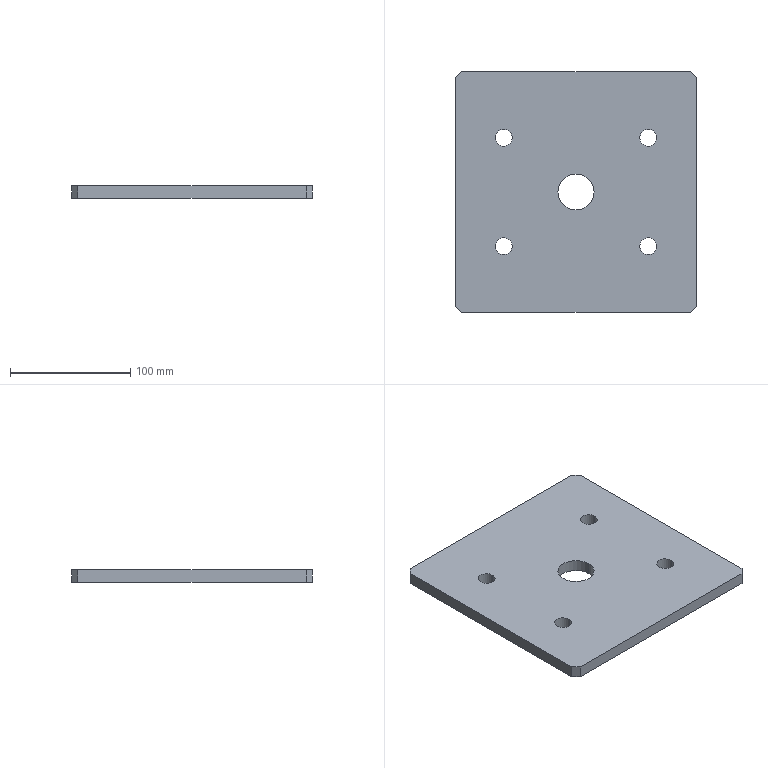Part | SolidWorks | features Chamfer 1, Extrusion 1, ICE 1 | 1 solid | 20 faces | box 200 x 200 x 10 mm | volume 386274 mm3 | cylinder 10 | plane 10 | commonest cylinder face diameters 14 x8 30 x2
STEP:
#1=CARTESIAN_POINT('',(85.,-100.,0.));
#2=VERTEX_POINT('',#1);
#3=CARTESIAN_POINT('',(115.,-100.,0.));
#4=VERTEX_POINT('',#3);
#5=CARTESIAN_POINT('',(100.,-100.,0.));
#6=DIRECTION('',(0.,0.,1.));
#7=DIRECTION('',(1.,0.,0.));
#8=AXIS2_PLACEMENT_3D('',#5,#6,#7);
#9=CIRCLE('',#8,15.);
#10=EDGE_CURVE('',#2,#4,#9,.T.);
#11=ORIENTED_EDGE('',*,*,#10,.F.);
#12=CARTESIAN_POINT('',(85.,-100.,10.));
#13=VERTEX_POINT('',#12);
#14=CARTESIAN_POINT('',(85.,-100.,0.));
#15=DIRECTION('',(0.,0.,1.));
#16=VECTOR('',#15,1000.);
#17=LINE('',#14,#16);
#18=EDGE_CURVE('',#2,#13,#17,.T.);
#19=ORIENTED_EDGE('',*,*,#18,.T.);
#20=CARTESIAN_POINT('',(115.,-100.,10.));
#21=VERTEX_POINT('',#20);
#22=CARTESIAN_POINT('',(100.,-100.,10.));
#23=DIRECTION('',(0.,0.,1.));
#24=DIRECTION('',(1.,0.,0.));
#25=AXIS2_PLACEMENT_3D('',#22,#23,#24);
#26=CIRCLE('',#25,15.);
#27=EDGE_CURVE('',#13,#21,#26,.T.);
#28=ORIENTED_EDGE('',*,*,#27,.T.);
#29=CARTESIAN_POINT('',(115.,-100.,0.));
#30=DIRECTION('',(0.,0.,1.));
#31=VECTOR('',#30,1000.);
#32=LINE('',#29,#31);
#33=EDGE_CURVE('',#4,#21,#32,.T.);
#34=ORIENTED_EDGE('',*,*,#33,.F.);
#35=EDGE_LOOP('',(#11,#19,#28,#34));
#36=FACE_OUTER_BOUND('',#35,.T.);
#37=CARTESIAN_POINT('',(100.,-100.,0.));
#38=DIRECTION('',(0.,0.,1.));
#39=DIRECTION('',(1.,0.,0.));
#40=AXIS2_PLACEMENT_3D('',#37,#38,#39);
#41=CYLINDRICAL_SURFACE('',#40,15.);
#42=ADVANCED_FACE('',(#36),#41,.F.);
#43=CARTESIAN_POINT('',(153.,-55.,0.));
#44=VERTEX_POINT('',#43);
#45=CARTESIAN_POINT('',(167.,-55.,0.));
#46=VERTEX_POINT('',#45);
#47=CARTESIAN_POINT('',(160.,-55.,0.));
#48=DIRECTION('',(0.,0.,1.));
#49=DIRECTION('',(1.,0.,0.));
#50=AXIS2_PLACEMENT_3D('',#47,#48,#49);
#51=CIRCLE('',#50,7.);
#52=EDGE_CURVE('',#44,#46,#51,.T.);
#53=ORIENTED_EDGE('',*,*,#52,.F.);
#54=CARTESIAN_POINT('',(153.,-55.,10.));
#55=VERTEX_POINT('',#54);
#56=CARTESIAN_POINT('',(153.,-55.,0.));
#57=DIRECTION('',(0.,0.,1.));
#58=VECTOR('',#57,1000.);
#59=LINE('',#56,#58);
#60=EDGE_CURVE('',#44,#55,#59,.T.);
#61=ORIENTED_EDGE('',*,*,#60,.T.);
#62=CARTESIAN_POINT('',(167.,-55.,10.));
#63=VERTEX_POINT('',#62);
#64=CARTESIAN_POINT('',(160.,-55.,10.));
#65=DIRECTION('',(0.,0.,1.));
#66=DIRECTION('',(1.,0.,0.));
#67=AXIS2_PLACEMENT_3D('',#64,#65,#66);
#68=CIRCLE('',#67,7.);
#69=EDGE_CURVE('',#55,#63,#68,.T.);
#70=ORIENTED_EDGE('',*,*,#69,.T.);
#71=CARTESIAN_POINT('',(167.,-55.,0.));
#72=DIRECTION('',(0.,0.,1.));
#73=VECTOR('',#72,1000.);
#74=LINE('',#71,#73);
#75=EDGE_CURVE('',#46,#63,#74,.T.);
#76=ORIENTED_EDGE('',*,*,#75,.F.);
#77=EDGE_LOOP('',(#53,#61,#70,#76));
#78=FACE_OUTER_BOUND('',#77,.T.);
#79=CARTESIAN_POINT('',(160.,-55.,0.));
#80=DIRECTION('',(0.,0.,1.));
#81=DIRECTION('',(1.,0.,0.));
#82=AXIS2_PLACEMENT_3D('',#79,#80,#81);
#83=CYLINDRICAL_SURFACE('',#82,7.);
#84=ADVANCED_FACE('',(#78),#83,.F.);
#85=CARTESIAN_POINT('',(153.,-145.,0.));
#86=VERTEX_POINT('',#85);
#87=CARTESIAN_POINT('',(167.,-145.,0.));
#88=VERTEX_POINT('',#87);
#89=CARTESIAN_POINT('',(160.,-145.,0.));
#90=DIRECTION('',(0.,0.,1.));
#91=DIRECTION('',(1.,0.,0.));
#92=AXIS2_PLACEMENT_3D('',#89,#90,#91);
#93=CIRCLE('',#92,7.);
#94=EDGE_CURVE('',#86,#88,#93,.T.);
#95=ORIENTED_EDGE('',*,*,#94,.F.);
#96=CARTESIAN_POINT('',(153.,-145.,10.));
#97=VERTEX_POINT('',#96);
#98=CARTESIAN_POINT('',(153.,-145.,0.));
#99=DIRECTION('',(0.,0.,1.));
#100=VECTOR('',#99,1000.);
#101=LINE('',#98,#100);
#102=EDGE_CURVE('',#86,#97,#101,.T.);
#103=ORIENTED_EDGE('',*,*,#102,.T.);
#104=CARTESIAN_POINT('',(167.,-145.,10.));
#105=VERTEX_POINT('',#104);
#106=CARTESIAN_POINT('',(160.,-145.,10.));
#107=DIRECTION('',(0.,0.,1.));
#108=DIRECTION('',(1.,0.,0.));
#109=AXIS2_PLACEMENT_3D('',#106,#107,#108);
#110=CIRCLE('',#109,7.);
#111=EDGE_CURVE('',#97,#105,#110,.T.);
#112=ORIENTED_EDGE('',*,*,#111,.T.);
#113=CARTESIAN_POINT('',(167.,-145.,0.));
#114=DIRECTION('',(0.,0.,1.));
#115=VECTOR('',#114,1000.);
#116=LINE('',#113,#115);
#117=EDGE_CURVE('',#88,#105,#116,.T.);
#118=ORIENTED_EDGE('',*,*,#117,.F.);
#119=EDGE_LOOP('',(#95,#103,#112,#118));
#120=FACE_OUTER_BOUND('',#119,.T.);
#121=CARTESIAN_POINT('',(160.,-145.,0.));
#122=DIRECTION('',(0.,0.,1.));
#123=DIRECTION('',(1.,0.,0.));
#124=AXIS2_PLACEMENT_3D('',#121,#122,#123);
#125=CYLINDRICAL_SURFACE('',#124,7.);
#126=ADVANCED_FACE('',(#120),#125,.F.);
#127=CARTESIAN_POINT('',(33.,-145.,0.));
#128=VERTEX_POINT('',#127);
#129=CARTESIAN_POINT('',(47.,-145.,0.));
#130=VERTEX_POINT('',#129);
#131=CARTESIAN_POINT('',(40.,-145.,0.));
#132=DIRECTION('',(0.,0.,1.));
#133=DIRECTION('',(1.,0.,0.));
#134=AXIS2_PLACEMENT_3D('',#131,#132,#133);
#135=CIRCLE('',#134,7.);
#136=EDGE_CURVE('',#128,#130,#135,.T.);
#137=ORIENTED_EDGE('',*,*,#136,.F.);
#138=CARTESIAN_POINT('',(33.,-145.,10.));
#139=VERTEX_POINT('',#138);
#140=CARTESIAN_POINT('',(33.,-145.,0.));
#141=DIRECTION('',(0.,0.,1.));
#142=VECTOR('',#141,1000.);
#143=LINE('',#140,#142);
#144=EDGE_CURVE('',#128,#139,#143,.T.);
#145=ORIENTED_EDGE('',*,*,#144,.T.);
#146=CARTESIAN_POINT('',(47.,-145.,10.));
#147=VERTEX_POINT('',#146);
#148=CARTESIAN_POINT('',(40.,-145.,10.));
#149=DIRECTION('',(0.,0.,1.));
#150=DIRECTION('',(1.,0.,0.));
#151=AXIS2_PLACEMENT_3D('',#148,#149,#150);
#152=CIRCLE('',#151,7.);
#153=EDGE_CURVE('',#139,#147,#152,.T.);
#154=ORIENTED_EDGE('',*,*,#153,.T.);
#155=CARTESIAN_POINT('',(47.,-145.,0.));
#156=DIRECTION('',(0.,0.,1.));
#157=VECTOR('',#156,1000.);
#158=LINE('',#155,#157);
#159=EDGE_CURVE('',#130,#147,#158,.T.);
#160=ORIENTED_EDGE('',*,*,#159,.F.);
#161=EDGE_LOOP('',(#137,#145,#154,#160));
#162=FACE_OUTER_BOUND('',#161,.T.);
#163=CARTESIAN_POINT('',(40.,-145.,0.));
#164=DIRECTION('',(0.,0.,1.));
#165=DIRECTION('',(1.,0.,0.));
#166=AXIS2_PLACEMENT_3D('',#163,#164,#165);
#167=CYLINDRICAL_SURFACE('',#166,7.);
#168=ADVANCED_FACE('',(#162),#167,.F.);
#169=CARTESIAN_POINT('',(33.,-55.,0.));
#170=VERTEX_POINT('',#169);
#171=CARTESIAN_POINT('',(47.,-55.,0.));
#172=VERTEX_POINT('',#171);
#173=CARTESIAN_POINT('',(40.,-55.,0.));
#174=DIRECTION('',(0.,0.,1.));
#175=DIRECTION('',(1.,0.,0.));
#176=AXIS2_PLACEMENT_3D('',#173,#174,#175);
#177=CIRCLE('',#176,7.);
#178=EDGE_CURVE('',#170,#172,#177,.T.);
#179=ORIENTED_EDGE('',*,*,#178,.F.);
#180=CARTESIAN_POINT('',(33.,-55.,10.));
#181=VERTEX_POINT('',#180);
#182=CARTESIAN_POINT('',(33.,-55.,0.));
#183=DIRECTION('',(0.,0.,1.));
#184=VECTOR('',#183,1000.);
#185=LINE('',#182,#184);
#186=EDGE_CURVE('',#170,#181,#185,.T.);
#187=ORIENTED_EDGE('',*,*,#186,.T.);
#188=CARTESIAN_POINT('',(47.,-55.,10.));
#189=VERTEX_POINT('',#188);
#190=CARTESIAN_POINT('',(40.,-55.,10.));
#191=DIRECTION('',(0.,0.,1.));
#192=DIRECTION('',(1.,0.,0.));
#193=AXIS2_PLACEMENT_3D('',#190,#191,#192);
#194=CIRCLE('',#193,7.);
#195=EDGE_CURVE('',#181,#189,#194,.T.);
#196=ORIENTED_EDGE('',*,*,#195,.T.);
#197=CARTESIAN_POINT('',(47.,-55.,0.));
#198=DIRECTION('',(0.,0.,1.));
#199=VECTOR('',#198,1000.);
#200=LINE('',#197,#199);
#201=EDGE_CURVE('',#172,#189,#200,.T.);
#202=ORIENTED_EDGE('',*,*,#201,.F.);
#203=EDGE_LOOP('',(#179,#187,#196,#202));
#204=FACE_OUTER_BOUND('',#203,.T.);
#205=CARTESIAN_POINT('',(40.,-55.,0.));
#206=DIRECTION('',(0.,0.,1.));
#207=DIRECTION('',(1.,0.,0.));
#208=AXIS2_PLACEMENT_3D('',#205,#206,#207);
#209=CYLINDRICAL_SURFACE('',#208,7.);
#210=ADVANCED_FACE('',(#204),#209,.F.);
#211=CARTESIAN_POINT('',(0.,-5.,0.));
#212=VERTEX_POINT('',#211);
#213=CARTESIAN_POINT('',(0.,-195.,0.));
#214=VERTEX_POINT('',#213);
#215=CARTESIAN_POINT('',(0.,0.,0.));
#216=DIRECTION('',(0.,-1.,0.));
#217=VECTOR('',#216,1000.);
#218=LINE('',#215,#217);
#219=EDGE_CURVE('',#212,#214,#218,.T.);
#220=ORIENTED_EDGE('',*,*,#219,.T.);
#221=CARTESIAN_POINT('',(0.,-195.,10.));
#222=VERTEX_POINT('',#221);
#223=CARTESIAN_POINT('',(0.,-195.,10.));
#224=DIRECTION('',(0.,0.,1.));
#225=VECTOR('',#224,1000.);
#226=LINE('',#223,#225);
#227=EDGE_CURVE('',#214,#222,#226,.T.);
#228=ORIENTED_EDGE('',*,*,#227,.T.);
#229=CARTESIAN_POINT('',(0.,-5.,10.));
#230=VERTEX_POINT('',#229);
#231=CARTESIAN_POINT('',(0.,0.,10.));
#232=DIRECTION('',(0.,-1.,0.));
#233=VECTOR('',#232,1000.);
#234=LINE('',#231,#233);
#235=EDGE_CURVE('',#230,#222,#234,.T.);
#236=ORIENTED_EDGE('',*,*,#235,.F.);
#237=CARTESIAN_POINT('',(0.,-5.,10.));
#238=DIRECTION('',(0.,0.,-1.));
#239=VECTOR('',#238,1000.);
#240=LINE('',#237,#239);
#241=EDGE_CURVE('',#230,#212,#240,.T.);
#242=ORIENTED_EDGE('',*,*,#241,.T.);
#243=EDGE_LOOP('',(#220,#228,#236,#242));
#244=FACE_OUTER_BOUND('',#243,.T.);
#245=CARTESIAN_POINT('',(0.,0.,10.));
#246=DIRECTION('',(1.,0.,0.));
#247=DIRECTION('',(0.,1.,0.));
#248=AXIS2_PLACEMENT_3D('',#245,#246,#247);
#249=PLANE('',#248);
#250=ADVANCED_FACE('',(#244),#249,.F.);
#251=CARTESIAN_POINT('',(5.,-200.,10.));
#252=VERTEX_POINT('',#251);
#253=CARTESIAN_POINT('',(195.,-200.,10.));
#254=VERTEX_POINT('',#253);
#255=CARTESIAN_POINT('',(0.,-200.,10.));
#256=DIRECTION('',(1.,0.,0.));
#257=VECTOR('',#256,1000.);
#258=LINE('',#255,#257);
#259=EDGE_CURVE('',#252,#254,#258,.T.);
#260=ORIENTED_EDGE('',*,*,#259,.F.);
#261=CARTESIAN_POINT('',(5.,-200.,0.));
#262=VERTEX_POINT('',#261);
#263=CARTESIAN_POINT('',(5.,-200.,10.));
#264=DIRECTION('',(0.,0.,-1.));
#265=VECTOR('',#264,1000.);
#266=LINE('',#263,#265);
#267=EDGE_CURVE('',#252,#262,#266,.T.);
#268=ORIENTED_EDGE('',*,*,#267,.T.);
#269=CARTESIAN_POINT('',(195.,-200.,0.));
#270=VERTEX_POINT('',#269);
#271=CARTESIAN_POINT('',(0.,-200.,0.));
#272=DIRECTION('',(1.,0.,0.));
#273=VECTOR('',#272,1000.);
#274=LINE('',#271,#273);
#275=EDGE_CURVE('',#262,#270,#274,.T.);
#276=ORIENTED_EDGE('',*,*,#275,.T.);
#277=CARTESIAN_POINT('',(195.,-200.,10.));
#278=DIRECTION('',(0.,0.,1.));
#279=VECTOR('',#278,1000.);
#280=LINE('',#277,#279);
#281=EDGE_CURVE('',#270,#254,#280,.T.);
#282=ORIENTED_EDGE('',*,*,#281,.T.);
#283=EDGE_LOOP('',(#260,#268,#276,#282));
#284=FACE_OUTER_BOUND('',#283,.T.);
#285=CARTESIAN_POINT('',(0.,-200.,10.));
#286=DIRECTION('',(0.,1.,0.));
#287=DIRECTION('',(0.,0.,1.));
#288=AXIS2_PLACEMENT_3D('',#285,#286,#287);
#289=PLANE('',#288);
#290=ADVANCED_FACE('',(#284),#289,.F.);
#291=CARTESIAN_POINT('',(200.,-195.,10.));
#292=VERTEX_POINT('',#291);
#293=CARTESIAN_POINT('',(200.,-5.,10.));
#294=VERTEX_POINT('',#293);
#295=CARTESIAN_POINT('',(200.,0.,10.));
#296=DIRECTION('',(0.,1.,0.));
#297=VECTOR('',#296,1000.);
#298=LINE('',#295,#297);
#299=EDGE_CURVE('',#292,#294,#298,.T.);
#300=ORIENTED_EDGE('',*,*,#299,.F.);
#301=CARTESIAN_POINT('',(200.,-195.,0.));
#302=VERTEX_POINT('',#301);
#303=CARTESIAN_POINT('',(200.,-195.,10.));
#304=DIRECTION('',(0.,0.,-1.));
#305=VECTOR('',#304,1000.);
#306=LINE('',#303,#305);
#307=EDGE_CURVE('',#292,#302,#306,.T.);
#308=ORIENTED_EDGE('',*,*,#307,.T.);
#309=CARTESIAN_POINT('',(200.,-5.,0.));
#310=VERTEX_POINT('',#309);
#311=CARTESIAN_POINT('',(200.,0.,0.));
#312=DIRECTION('',(0.,1.,0.));
#313=VECTOR('',#312,1000.);
#314=LINE('',#311,#313);
#315=EDGE_CURVE('',#302,#310,#314,.T.);
#316=ORIENTED_EDGE('',*,*,#315,.T.);
#317=CARTESIAN_POINT('',(200.,-5.,10.));
#318=DIRECTION('',(0.,0.,1.));
#319=VECTOR('',#318,1000.);
#320=LINE('',#317,#319);
#321=EDGE_CURVE('',#310,#294,#320,.T.);
#322=ORIENTED_EDGE('',*,*,#321,.T.);
#323=EDGE_LOOP('',(#300,#308,#316,#322));
#324=FACE_OUTER_BOUND('',#323,.T.);
#325=CARTESIAN_POINT('',(200.,0.,10.));
#326=DIRECTION('',(-1.,0.,0.));
#327=DIRECTION('',(0.,-1.,0.));
#328=AXIS2_PLACEMENT_3D('',#325,#326,#327);
#329=PLANE('',#328);
#330=ADVANCED_FACE('',(#324),#329,.F.);
#331=CARTESIAN_POINT('',(195.,0.,10.));
#332=VERTEX_POINT('',#331);
#333=CARTESIAN_POINT('',(5.,0.,10.));
#334=VERTEX_POINT('',#333);
#335=CARTESIAN_POINT('',(0.,0.,10.));
#336=DIRECTION('',(-1.,0.,0.));
#337=VECTOR('',#336,1000.);
#338=LINE('',#335,#337);
#339=EDGE_CURVE('',#332,#334,#338,.T.);
#340=ORIENTED_EDGE('',*,*,#339,.F.);
#341=CARTESIAN_POINT('',(195.,0.,0.));
#342=VERTEX_POINT('',#341);
#343=CARTESIAN_POINT('',(195.,0.,10.));
#344=DIRECTION('',(0.,0.,-1.));
#345=VECTOR('',#344,1000.);
#346=LINE('',#343,#345);
#347=EDGE_CURVE('',#332,#342,#346,.T.);
#348=ORIENTED_EDGE('',*,*,#347,.T.);
#349=CARTESIAN_POINT('',(5.,0.,0.));
#350=VERTEX_POINT('',#349);
#351=CARTESIAN_POINT('',(0.,0.,0.));
#352=DIRECTION('',(-1.,0.,0.));
#353=VECTOR('',#352,1000.);
#354=LINE('',#351,#353);
#355=EDGE_CURVE('',#342,#350,#354,.T.);
#356=ORIENTED_EDGE('',*,*,#355,.T.);
#357=CARTESIAN_POINT('',(5.,0.,10.));
#358=DIRECTION('',(0.,0.,1.));
#359=VECTOR('',#358,1000.);
#360=LINE('',#357,#359);
#361=EDGE_CURVE('',#350,#334,#360,.T.);
#362=ORIENTED_EDGE('',*,*,#361,.T.);
#363=EDGE_LOOP('',(#340,#348,#356,#362));
#364=FACE_OUTER_BOUND('',#363,.T.);
#365=CARTESIAN_POINT('',(0.,0.,10.));
#366=DIRECTION('',(0.,-1.,0.));
#367=DIRECTION('',(0.,0.,-1.));
#368=AXIS2_PLACEMENT_3D('',#365,#366,#367);
#369=PLANE('',#368);
#370=ADVANCED_FACE('',(#364),#369,.F.);
#371=CARTESIAN_POINT('',(100.,-100.,10.));
#372=DIRECTION('',(0.,0.,1.));
#373=DIRECTION('',(1.,0.,0.));
#374=AXIS2_PLACEMENT_3D('',#371,#372,#373);
#375=CIRCLE('',#374,15.);
#376=EDGE_CURVE('',#21,#13,#375,.T.);
#377=ORIENTED_EDGE('',*,*,#376,.F.);
#378=ORIENTED_EDGE('',*,*,#27,.F.);
#379=EDGE_LOOP('',(#377,#378));
#380=FACE_BOUND('',#379,.T.);
#381=CARTESIAN_POINT('',(160.,-55.,10.));
#382=DIRECTION('',(0.,0.,1.));
#383=DIRECTION('',(1.,0.,0.));
#384=AXIS2_PLACEMENT_3D('',#381,#382,#383);
#385=CIRCLE('',#384,7.);
#386=EDGE_CURVE('',#63,#55,#385,.T.);
#387=ORIENTED_EDGE('',*,*,#386,.F.);
#388=ORIENTED_EDGE('',*,*,#69,.F.);
#389=EDGE_LOOP('',(#387,#388));
#390=FACE_BOUND('',#389,.T.);
#391=CARTESIAN_POINT('',(160.,-145.,10.));
#392=DIRECTION('',(0.,0.,1.));
#393=DIRECTION('',(1.,0.,0.));
#394=AXIS2_PLACEMENT_3D('',#391,#392,#393);
#395=CIRCLE('',#394,7.);
#396=EDGE_CURVE('',#105,#97,#395,.T.);
#397=ORIENTED_EDGE('',*,*,#396,.F.);
#398=ORIENTED_EDGE('',*,*,#111,.F.);
#399=EDGE_LOOP('',(#397,#398));
#400=FACE_BOUND('',#399,.T.);
#401=CARTESIAN_POINT('',(40.,-145.,10.));
#402=DIRECTION('',(0.,0.,1.));
#403=DIRECTION('',(1.,0.,0.));
#404=AXIS2_PLACEMENT_3D('',#401,#402,#403);
#405=CIRCLE('',#404,7.);
#406=EDGE_CURVE('',#147,#139,#405,.T.);
#407=ORIENTED_EDGE('',*,*,#406,.F.);
#408=ORIENTED_EDGE('',*,*,#153,.F.);
#409=EDGE_LOOP('',(#407,#408));
#410=FACE_BOUND('',#409,.T.);
#411=CARTESIAN_POINT('',(40.,-55.,10.));
#412=DIRECTION('',(0.,0.,1.));
#413=DIRECTION('',(1.,0.,0.));
#414=AXIS2_PLACEMENT_3D('',#411,#412,#413);
#415=CIRCLE('',#414,7.);
#416=EDGE_CURVE('',#189,#181,#415,.T.);
#417=ORIENTED_EDGE('',*,*,#416,.F.);
#418=ORIENTED_EDGE('',*,*,#195,.F.);
#419=EDGE_LOOP('',(#417,#418));
#420=FACE_BOUND('',#419,.T.);
#421=ORIENTED_EDGE('',*,*,#235,.T.);
#422=CARTESIAN_POINT('',(-97.5,-97.5,10.));
#423=DIRECTION('',(0.7071,-0.7071,0.));
#424=VECTOR('',#423,1000.);
#425=LINE('',#422,#424);
#426=EDGE_CURVE('',#222,#252,#425,.T.);
#427=ORIENTED_EDGE('',*,*,#426,.T.);
#428=ORIENTED_EDGE('',*,*,#259,.T.);
#429=CARTESIAN_POINT('',(197.5,-197.5,10.));
#430=DIRECTION('',(0.7071,0.7071,0.));
#431=VECTOR('',#430,1000.);
#432=LINE('',#429,#431);
#433=EDGE_CURVE('',#254,#292,#432,.T.);
#434=ORIENTED_EDGE('',*,*,#433,.T.);
#435=ORIENTED_EDGE('',*,*,#299,.T.);
#436=CARTESIAN_POINT('',(97.5,97.5,10.));
#437=DIRECTION('',(-0.7071,0.7071,0.));
#438=VECTOR('',#437,1000.);
#439=LINE('',#436,#438);
#440=EDGE_CURVE('',#294,#332,#439,.T.);
#441=ORIENTED_EDGE('',*,*,#440,.T.);
#442=ORIENTED_EDGE('',*,*,#339,.T.);
#443=CARTESIAN_POINT('',(2.5,-2.5,10.));
#444=DIRECTION('',(-0.7071,-0.7071,0.));
#445=VECTOR('',#444,1000.);
#446=LINE('',#443,#445);
#447=EDGE_CURVE('',#334,#230,#446,.T.);
#448=ORIENTED_EDGE('',*,*,#447,.T.);
#449=EDGE_LOOP('',(#421,#427,#428,#434,#435,#441,#442,#448));
#450=FACE_OUTER_BOUND('',#449,.T.);
#451=CARTESIAN_POINT('',(0.,0.,10.));
#452=DIRECTION('',(0.,0.,1.));
#453=DIRECTION('',(1.,0.,0.));
#454=AXIS2_PLACEMENT_3D('',#451,#452,#453);
#455=PLANE('',#454);
#456=ADVANCED_FACE('',(#380,#390,#400,#410,#420,#450),#455,.T.);
#457=CARTESIAN_POINT('',(100.,-100.,0.));
#458=DIRECTION('',(0.,0.,1.));
#459=DIRECTION('',(1.,0.,0.));
#460=AXIS2_PLACEMENT_3D('',#457,#458,#459);
#461=CIRCLE('',#460,15.);
#462=EDGE_CURVE('',#4,#2,#461,.T.);
#463=ORIENTED_EDGE('',*,*,#462,.T.);
#464=ORIENTED_EDGE('',*,*,#10,.T.);
#465=EDGE_LOOP('',(#463,#464));
#466=FACE_BOUND('',#465,.T.);
#467=CARTESIAN_POINT('',(160.,-55.,0.));
#468=DIRECTION('',(0.,0.,1.));
#469=DIRECTION('',(1.,0.,0.));
#470=AXIS2_PLACEMENT_3D('',#467,#468,#469);
#471=CIRCLE('',#470,7.);
#472=EDGE_CURVE('',#46,#44,#471,.T.);
#473=ORIENTED_EDGE('',*,*,#472,.T.);
#474=ORIENTED_EDGE('',*,*,#52,.T.);
#475=EDGE_LOOP('',(#473,#474));
#476=FACE_BOUND('',#475,.T.);
#477=CARTESIAN_POINT('',(160.,-145.,0.));
#478=DIRECTION('',(0.,0.,1.));
#479=DIRECTION('',(1.,0.,0.));
#480=AXIS2_PLACEMENT_3D('',#477,#478,#479);
#481=CIRCLE('',#480,7.);
#482=EDGE_CURVE('',#88,#86,#481,.T.);
#483=ORIENTED_EDGE('',*,*,#482,.T.);
#484=ORIENTED_EDGE('',*,*,#94,.T.);
#485=EDGE_LOOP('',(#483,#484));
#486=FACE_BOUND('',#485,.T.);
#487=CARTESIAN_POINT('',(40.,-145.,0.));
#488=DIRECTION('',(0.,0.,1.));
#489=DIRECTION('',(1.,0.,0.));
#490=AXIS2_PLACEMENT_3D('',#487,#488,#489);
#491=CIRCLE('',#490,7.);
#492=EDGE_CURVE('',#130,#128,#491,.T.);
#493=ORIENTED_EDGE('',*,*,#492,.T.);
#494=ORIENTED_EDGE('',*,*,#136,.T.);
#495=EDGE_LOOP('',(#493,#494));
#496=FACE_BOUND('',#495,.T.);
#497=CARTESIAN_POINT('',(40.,-55.,0.));
#498=DIRECTION('',(0.,0.,1.));
#499=DIRECTION('',(1.,0.,0.));
#500=AXIS2_PLACEMENT_3D('',#497,#498,#499);
#501=CIRCLE('',#500,7.);
#502=EDGE_CURVE('',#172,#170,#501,.T.);
#503=ORIENTED_EDGE('',*,*,#502,.T.);
#504=ORIENTED_EDGE('',*,*,#178,.T.);
#505=EDGE_LOOP('',(#503,#504));
#506=FACE_BOUND('',#505,.T.);
#507=ORIENTED_EDGE('',*,*,#275,.F.);
#508=CARTESIAN_POINT('',(5.,-200.,0.));
#509=DIRECTION('',(-0.7071,0.7071,0.));
#510=VECTOR('',#509,1000.);
#511=LINE('',#508,#510);
#512=EDGE_CURVE('',#262,#214,#511,.T.);
#513=ORIENTED_EDGE('',*,*,#512,.T.);
#514=ORIENTED_EDGE('',*,*,#219,.F.);
#515=CARTESIAN_POINT('',(0.,-5.,0.));
#516=DIRECTION('',(0.7071,0.7071,0.));
#517=VECTOR('',#516,1000.);
#518=LINE('',#515,#517);
#519=EDGE_CURVE('',#212,#350,#518,.T.);
#520=ORIENTED_EDGE('',*,*,#519,.T.);
#521=ORIENTED_EDGE('',*,*,#355,.F.);
#522=CARTESIAN_POINT('',(195.,0.,0.));
#523=DIRECTION('',(0.7071,-0.7071,0.));
#524=VECTOR('',#523,1000.);
#525=LINE('',#522,#524);
#526=EDGE_CURVE('',#342,#310,#525,.T.);
#527=ORIENTED_EDGE('',*,*,#526,.T.);
#528=ORIENTED_EDGE('',*,*,#315,.F.);
#529=CARTESIAN_POINT('',(200.,-195.,0.));
#530=DIRECTION('',(-0.7071,-0.7071,0.));
#531=VECTOR('',#530,1000.);
#532=LINE('',#529,#531);
#533=EDGE_CURVE('',#302,#270,#532,.T.);
#534=ORIENTED_EDGE('',*,*,#533,.T.);
#535=EDGE_LOOP('',(#507,#513,#514,#520,#521,#527,#528,#534));
#536=FACE_OUTER_BOUND('',#535,.T.);
#537=CARTESIAN_POINT('',(0.,0.,0.));
#538=DIRECTION('',(0.,0.,1.));
#539=DIRECTION('',(1.,0.,0.));
#540=AXIS2_PLACEMENT_3D('',#537,#538,#539);
#541=PLANE('',#540);
#542=ADVANCED_FACE('',(#466,#476,#486,#496,#506,#536),#541,.F.);
#543=ORIENTED_EDGE('',*,*,#186,.F.);
#544=ORIENTED_EDGE('',*,*,#502,.F.);
#545=ORIENTED_EDGE('',*,*,#201,.T.);
#546=ORIENTED_EDGE('',*,*,#416,.T.);
#547=EDGE_LOOP('',(#543,#544,#545,#546));
#548=FACE_OUTER_BOUND('',#547,.T.);
#549=CARTESIAN_POINT('',(40.,-55.,0.));
#550=DIRECTION('',(0.,0.,1.));
#551=DIRECTION('',(1.,0.,0.));
#552=AXIS2_PLACEMENT_3D('',#549,#550,#551);
#553=CYLINDRICAL_SURFACE('',#552,7.);
#554=ADVANCED_FACE('',(#548),#553,.F.);
#555=ORIENTED_EDGE('',*,*,#144,.F.);
#556=ORIENTED_EDGE('',*,*,#492,.F.);
#557=ORIENTED_EDGE('',*,*,#159,.T.);
#558=ORIENTED_EDGE('',*,*,#406,.T.);
#559=EDGE_LOOP('',(#555,#556,#557,#558));
#560=FACE_OUTER_BOUND('',#559,.T.);
#561=CARTESIAN_POINT('',(40.,-145.,0.));
#562=DIRECTION('',(0.,0.,1.));
#563=DIRECTION('',(1.,0.,0.));
#564=AXIS2_PLACEMENT_3D('',#561,#562,#563);
#565=CYLINDRICAL_SURFACE('',#564,7.);
#566=ADVANCED_FACE('',(#560),#565,.F.);
#567=ORIENTED_EDGE('',*,*,#102,.F.);
#568=ORIENTED_EDGE('',*,*,#482,.F.);
#569=ORIENTED_EDGE('',*,*,#117,.T.);
#570=ORIENTED_EDGE('',*,*,#396,.T.);
#571=EDGE_LOOP('',(#567,#568,#569,#570));
#572=FACE_OUTER_BOUND('',#571,.T.);
#573=CARTESIAN_POINT('',(160.,-145.,0.));
#574=DIRECTION('',(0.,0.,1.));
#575=DIRECTION('',(1.,0.,0.));
#576=AXIS2_PLACEMENT_3D('',#573,#574,#575);
#577=CYLINDRICAL_SURFACE('',#576,7.);
#578=ADVANCED_FACE('',(#572),#577,.F.);
#579=ORIENTED_EDGE('',*,*,#60,.F.);
#580=ORIENTED_EDGE('',*,*,#472,.F.);
#581=ORIENTED_EDGE('',*,*,#75,.T.);
#582=ORIENTED_EDGE('',*,*,#386,.T.);
#583=EDGE_LOOP('',(#579,#580,#581,#582));
#584=FACE_OUTER_BOUND('',#583,.T.);
#585=CARTESIAN_POINT('',(160.,-55.,0.));
#586=DIRECTION('',(0.,0.,1.));
#587=DIRECTION('',(1.,0.,0.));
#588=AXIS2_PLACEMENT_3D('',#585,#586,#587);
#589=CYLINDRICAL_SURFACE('',#588,7.);
#590=ADVANCED_FACE('',(#584),#589,.F.);
#591=ORIENTED_EDGE('',*,*,#18,.F.);
#592=ORIENTED_EDGE('',*,*,#462,.F.);
#593=ORIENTED_EDGE('',*,*,#33,.T.);
#594=ORIENTED_EDGE('',*,*,#376,.T.);
#595=EDGE_LOOP('',(#591,#592,#593,#594));
#596=FACE_OUTER_BOUND('',#595,.T.);
#597=CARTESIAN_POINT('',(100.,-100.,0.));
#598=DIRECTION('',(0.,0.,1.));
#599=DIRECTION('',(1.,0.,0.));
#600=AXIS2_PLACEMENT_3D('',#597,#598,#599);
#601=CYLINDRICAL_SURFACE('',#600,15.);
#602=ADVANCED_FACE('',(#596),#601,.F.);
#603=ORIENTED_EDGE('',*,*,#426,.F.);
#604=ORIENTED_EDGE('',*,*,#227,.F.);
#605=ORIENTED_EDGE('',*,*,#512,.F.);
#606=ORIENTED_EDGE('',*,*,#267,.F.);
#607=EDGE_LOOP('',(#603,#604,#605,#606));
#608=FACE_OUTER_BOUND('',#607,.T.);
#609=CARTESIAN_POINT('',(5.,-200.,10.));
#610=DIRECTION('',(0.7071,0.7071,0.));
#611=DIRECTION('',(0.,0.,-1.));
#612=AXIS2_PLACEMENT_3D('',#609,#610,#611);
#613=PLANE('',#612);
#614=ADVANCED_FACE('',(#608),#613,.F.);
#615=ORIENTED_EDGE('',*,*,#433,.F.);
#616=ORIENTED_EDGE('',*,*,#281,.F.);
#617=ORIENTED_EDGE('',*,*,#533,.F.);
#618=ORIENTED_EDGE('',*,*,#307,.F.);
#619=EDGE_LOOP('',(#615,#616,#617,#618));
#620=FACE_OUTER_BOUND('',#619,.T.);
#621=CARTESIAN_POINT('',(200.,-195.,10.));
#622=DIRECTION('',(-0.7071,0.7071,0.));
#623=DIRECTION('',(0.,0.,-1.));
#624=AXIS2_PLACEMENT_3D('',#621,#622,#623);
#625=PLANE('',#624);
#626=ADVANCED_FACE('',(#620),#625,.F.);
#627=ORIENTED_EDGE('',*,*,#440,.F.);
#628=ORIENTED_EDGE('',*,*,#321,.F.);
#629=ORIENTED_EDGE('',*,*,#526,.F.);
#630=ORIENTED_EDGE('',*,*,#347,.F.);
#631=EDGE_LOOP('',(#627,#628,#629,#630));
#632=FACE_OUTER_BOUND('',#631,.T.);
#633=CARTESIAN_POINT('',(195.,0.,10.));
#634=DIRECTION('',(-0.7071,-0.7071,0.));
#635=DIRECTION('',(0.,0.,-1.));
#636=AXIS2_PLACEMENT_3D('',#633,#634,#635);
#637=PLANE('',#636);
#638=ADVANCED_FACE('',(#632),#637,.F.);
#639=ORIENTED_EDGE('',*,*,#447,.F.);
#640=ORIENTED_EDGE('',*,*,#361,.F.);
#641=ORIENTED_EDGE('',*,*,#519,.F.);
#642=ORIENTED_EDGE('',*,*,#241,.F.);
#643=EDGE_LOOP('',(#639,#640,#641,#642));
#644=FACE_OUTER_BOUND('',#643,.T.);
#645=CARTESIAN_POINT('',(0.,-5.,10.));
#646=DIRECTION('',(0.7071,-0.7071,0.));
#647=DIRECTION('',(0.,0.,-1.));
#648=AXIS2_PLACEMENT_3D('',#645,#646,#647);
#649=PLANE('',#648);
#650=ADVANCED_FACE('',(#644),#649,.F.);
#651=CLOSED_SHELL('',(#42,#84,#126,#168,#210,#250,#290,#330,#370,#456,#542,#554,#566,#578,#590,#602,#614,#626,#638,#650));
#652=MANIFOLD_SOLID_BREP('',#651);
#653=CARTESIAN_POINT('',(0.,0.,0.));
#654=DIRECTION('',(0.,0.,1.));
#655=DIRECTION('',(1.,0.,0.));
#656=AXIS2_PLACEMENT_3D('',#653,#654,#655);
#657=(LENGTH_UNIT()NAMED_UNIT(*)SI_UNIT(.MILLI.,.METRE.));
#658=UNCERTAINTY_MEASURE_WITH_UNIT(LENGTH_MEASURE(0.00001),#657,'','');
#659=(NAMED_UNIT(*)PLANE_ANGLE_UNIT()SI_UNIT($,.RADIAN.));
#660=(NAMED_UNIT(*)SI_UNIT($,.STERADIAN.)SOLID_ANGLE_UNIT());
#661=(GEOMETRIC_REPRESENTATION_CONTEXT(3)GLOBAL_UNCERTAINTY_ASSIGNED_CONTEXT((#658))GLOBAL_UNIT_ASSIGNED_CONTEXT((#657,#659,#660))REPRESENTATION_CONTEXT('',''));
#662=ADVANCED_BREP_SHAPE_REPRESENTATION('',(#652,#656),#661);